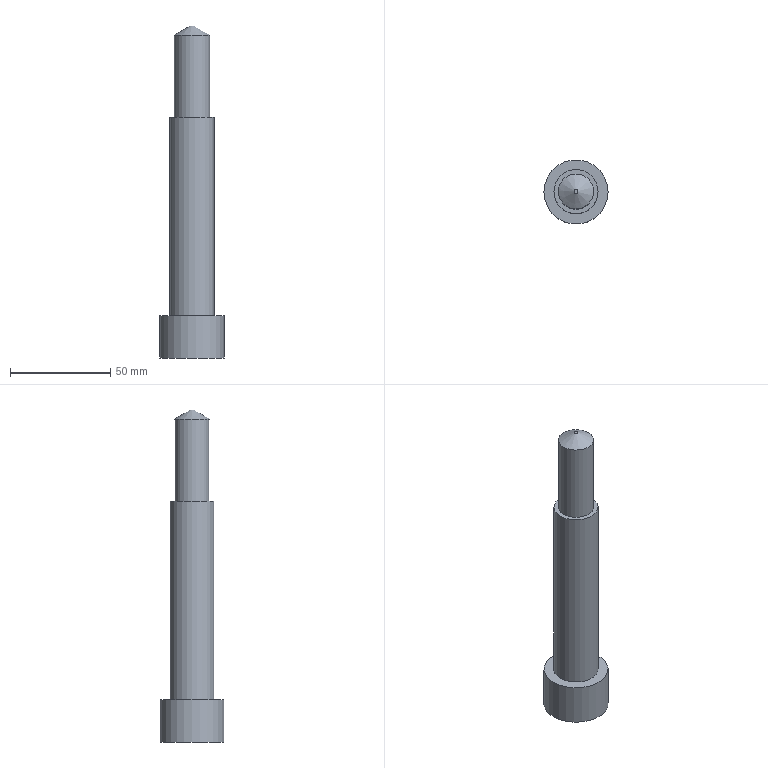Part | STEP file | solid 77 | 1 solid | 8 faces | box 32 x 32 x 165.5 mm | volume 64789 mm3 | plane 4 | cylinder 3 | cone 1 | commonest cylinder face diameters 17.5 x1 22 x1 32 x1